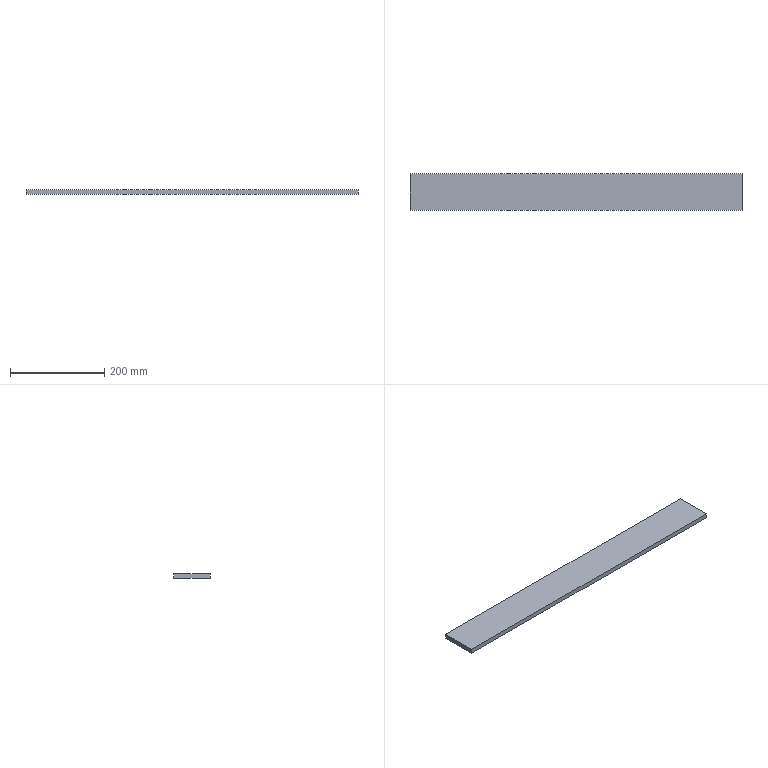Part | STEP file | 06-Square plate | 1 solid | 6 faces | box 703 x 78 x 10 mm | volume 548340 mm3 | plane 6
STEP:
#1=CARTESIAN_POINT('',(0.,0.,0.));
#2=DIRECTION('',(0.,0.,1.));
#3=DIRECTION('',(1.,0.,0.));
#4=AXIS2_PLACEMENT_3D('',#1,#2,#3);
#5=CARTESIAN_POINT('',(0.,0.,0.));
#6=VERTEX_POINT('',#5);
#7=CARTESIAN_POINT('',(0.,-78.,0.));
#8=VERTEX_POINT('',#7);
#9=CARTESIAN_POINT('',(0.,0.,0.));
#10=DIRECTION('',(0.,-1.,0.));
#11=VECTOR('',#10,1.);
#12=LINE('',#9,#11);
#13=CARTESIAN_POINT('',(0.,0.,10.));
#14=DIRECTION('',(1.,0.,0.));
#15=DIRECTION('',(0.,1.,0.));
#16=AXIS2_PLACEMENT_3D('',#13,#14,#15);
#17=PLANE('',#16);
#18=CARTESIAN_POINT('',(0.,-10.));
#19=DIRECTION('',(-1.,0.));
#20=VECTOR('',#19,1.);
#21=LINE('',#18,#20);
#22=(GEOMETRIC_REPRESENTATION_CONTEXT(2)PARAMETRIC_REPRESENTATION_CONTEXT()REPRESENTATION_CONTEXT('',''));
#23=DEFINITIONAL_REPRESENTATION('',(#21),#22);
#24=PCURVE('',#17,#23);
#25=CARTESIAN_POINT('',(0.,0.,0.));
#26=DIRECTION('',(0.,0.,1.));
#27=DIRECTION('',(1.,0.,0.));
#28=AXIS2_PLACEMENT_3D('',#25,#26,#27);
#29=PLANE('',#28);
#30=CARTESIAN_POINT('',(0.,0.));
#31=DIRECTION('',(0.,-1.));
#32=VECTOR('',#31,1.);
#33=LINE('',#30,#32);
#34=(GEOMETRIC_REPRESENTATION_CONTEXT(2)PARAMETRIC_REPRESENTATION_CONTEXT()REPRESENTATION_CONTEXT('',''));
#35=DEFINITIONAL_REPRESENTATION('',(#33),#34);
#36=PCURVE('',#29,#35);
#37=SURFACE_CURVE('',#12,(#24,#36),.PCURVE_S1.);
#38=EDGE_CURVE('',#6,#8,#37,.T.);
#39=ORIENTED_EDGE('',*,*,#38,.T.);
#40=CARTESIAN_POINT('',(0.,-78.,10.));
#41=VERTEX_POINT('',#40);
#42=CARTESIAN_POINT('',(0.,-78.,10.));
#43=DIRECTION('',(0.,0.,-1.));
#44=VECTOR('',#43,1.);
#45=LINE('',#42,#44);
#46=CARTESIAN_POINT('',(-78.,0.));
#47=DIRECTION('',(0.,-1.));
#48=VECTOR('',#47,1.);
#49=LINE('',#46,#48);
#50=(GEOMETRIC_REPRESENTATION_CONTEXT(2)PARAMETRIC_REPRESENTATION_CONTEXT()REPRESENTATION_CONTEXT('',''));
#51=DEFINITIONAL_REPRESENTATION('',(#49),#50);
#52=PCURVE('',#17,#51);
#53=CARTESIAN_POINT('',(0.,-78.,10.));
#54=DIRECTION('',(0.,1.,0.));
#55=DIRECTION('',(0.,0.,1.));
#56=AXIS2_PLACEMENT_3D('',#53,#54,#55);
#57=PLANE('',#56);
#58=CARTESIAN_POINT('',(0.,0.));
#59=DIRECTION('',(-1.,0.));
#60=VECTOR('',#59,1.);
#61=LINE('',#58,#60);
#62=(GEOMETRIC_REPRESENTATION_CONTEXT(2)PARAMETRIC_REPRESENTATION_CONTEXT()REPRESENTATION_CONTEXT('',''));
#63=DEFINITIONAL_REPRESENTATION('',(#61),#62);
#64=PCURVE('',#57,#63);
#65=SURFACE_CURVE('',#45,(#52,#64),.PCURVE_S1.);
#66=EDGE_CURVE('',#41,#8,#65,.T.);
#67=ORIENTED_EDGE('',*,*,#66,.F.);
#68=CARTESIAN_POINT('',(0.,0.,10.));
#69=VERTEX_POINT('',#68);
#70=CARTESIAN_POINT('',(0.,0.,10.));
#71=DIRECTION('',(0.,-1.,0.));
#72=VECTOR('',#71,1.);
#73=LINE('',#70,#72);
#74=CARTESIAN_POINT('',(0.,0.));
#75=DIRECTION('',(-1.,0.));
#76=VECTOR('',#75,1.);
#77=LINE('',#74,#76);
#78=(GEOMETRIC_REPRESENTATION_CONTEXT(2)PARAMETRIC_REPRESENTATION_CONTEXT()REPRESENTATION_CONTEXT('',''));
#79=DEFINITIONAL_REPRESENTATION('',(#77),#78);
#80=PCURVE('',#17,#79);
#81=CARTESIAN_POINT('',(0.,0.,10.));
#82=DIRECTION('',(0.,0.,1.));
#83=DIRECTION('',(1.,0.,0.));
#84=AXIS2_PLACEMENT_3D('',#81,#82,#83);
#85=PLANE('',#84);
#86=CARTESIAN_POINT('',(0.,0.));
#87=DIRECTION('',(0.,-1.));
#88=VECTOR('',#87,1.);
#89=LINE('',#86,#88);
#90=(GEOMETRIC_REPRESENTATION_CONTEXT(2)PARAMETRIC_REPRESENTATION_CONTEXT()REPRESENTATION_CONTEXT('',''));
#91=DEFINITIONAL_REPRESENTATION('',(#89),#90);
#92=PCURVE('',#85,#91);
#93=SURFACE_CURVE('',#73,(#80,#92),.PCURVE_S1.);
#94=EDGE_CURVE('',#69,#41,#93,.T.);
#95=ORIENTED_EDGE('',*,*,#94,.F.);
#96=CARTESIAN_POINT('',(0.,0.,10.));
#97=DIRECTION('',(0.,0.,-1.));
#98=VECTOR('',#97,1.);
#99=LINE('',#96,#98);
#100=CARTESIAN_POINT('',(0.,0.));
#101=DIRECTION('',(0.,-1.));
#102=VECTOR('',#101,1.);
#103=LINE('',#100,#102);
#104=(GEOMETRIC_REPRESENTATION_CONTEXT(2)PARAMETRIC_REPRESENTATION_CONTEXT()REPRESENTATION_CONTEXT('',''));
#105=DEFINITIONAL_REPRESENTATION('',(#103),#104);
#106=PCURVE('',#17,#105);
#107=CARTESIAN_POINT('',(0.,0.,10.));
#108=DIRECTION('',(0.,-1.,0.));
#109=DIRECTION('',(0.,0.,-1.));
#110=AXIS2_PLACEMENT_3D('',#107,#108,#109);
#111=PLANE('',#110);
#112=CARTESIAN_POINT('',(0.,0.));
#113=DIRECTION('',(1.,0.));
#114=VECTOR('',#113,1.);
#115=LINE('',#112,#114);
#116=(GEOMETRIC_REPRESENTATION_CONTEXT(2)PARAMETRIC_REPRESENTATION_CONTEXT()REPRESENTATION_CONTEXT('',''));
#117=DEFINITIONAL_REPRESENTATION('',(#115),#116);
#118=PCURVE('',#111,#117);
#119=SURFACE_CURVE('',#99,(#106,#118),.PCURVE_S1.);
#120=EDGE_CURVE('',#69,#6,#119,.T.);
#121=ORIENTED_EDGE('',*,*,#120,.T.);
#122=EDGE_LOOP('',(#39,#67,#95,#121));
#123=FACE_BOUND('',#122,.T.);
#124=ADVANCED_FACE('',(#123),#17,.F.);
#125=CARTESIAN_POINT('',(703.,-78.,0.));
#126=VERTEX_POINT('',#125);
#127=CARTESIAN_POINT('',(0.,-78.,0.));
#128=DIRECTION('',(1.,0.,0.));
#129=VECTOR('',#128,1.);
#130=LINE('',#127,#129);
#131=CARTESIAN_POINT('',(-10.,0.));
#132=DIRECTION('',(0.,1.));
#133=VECTOR('',#132,1.);
#134=LINE('',#131,#133);
#135=(GEOMETRIC_REPRESENTATION_CONTEXT(2)PARAMETRIC_REPRESENTATION_CONTEXT()REPRESENTATION_CONTEXT('',''));
#136=DEFINITIONAL_REPRESENTATION('',(#134),#135);
#137=PCURVE('',#57,#136);
#138=CARTESIAN_POINT('',(0.,-78.));
#139=DIRECTION('',(1.,0.));
#140=VECTOR('',#139,1.);
#141=LINE('',#138,#140);
#142=(GEOMETRIC_REPRESENTATION_CONTEXT(2)PARAMETRIC_REPRESENTATION_CONTEXT()REPRESENTATION_CONTEXT('',''));
#143=DEFINITIONAL_REPRESENTATION('',(#141),#142);
#144=PCURVE('',#29,#143);
#145=SURFACE_CURVE('',#130,(#137,#144),.PCURVE_S1.);
#146=EDGE_CURVE('',#8,#126,#145,.T.);
#147=ORIENTED_EDGE('',*,*,#146,.T.);
#148=CARTESIAN_POINT('',(703.,-78.,10.));
#149=VERTEX_POINT('',#148);
#150=CARTESIAN_POINT('',(703.,-78.,10.));
#151=DIRECTION('',(0.,0.,-1.));
#152=VECTOR('',#151,1.);
#153=LINE('',#150,#152);
#154=CARTESIAN_POINT('',(0.,703.));
#155=DIRECTION('',(-1.,0.));
#156=VECTOR('',#155,1.);
#157=LINE('',#154,#156);
#158=(GEOMETRIC_REPRESENTATION_CONTEXT(2)PARAMETRIC_REPRESENTATION_CONTEXT()REPRESENTATION_CONTEXT('',''));
#159=DEFINITIONAL_REPRESENTATION('',(#157),#158);
#160=PCURVE('',#57,#159);
#161=CARTESIAN_POINT('',(703.,0.,10.));
#162=DIRECTION('',(-1.,0.,0.));
#163=DIRECTION('',(0.,-1.,0.));
#164=AXIS2_PLACEMENT_3D('',#161,#162,#163);
#165=PLANE('',#164);
#166=CARTESIAN_POINT('',(78.,0.));
#167=DIRECTION('',(0.,-1.));
#168=VECTOR('',#167,1.);
#169=LINE('',#166,#168);
#170=(GEOMETRIC_REPRESENTATION_CONTEXT(2)PARAMETRIC_REPRESENTATION_CONTEXT()REPRESENTATION_CONTEXT('',''));
#171=DEFINITIONAL_REPRESENTATION('',(#169),#170);
#172=PCURVE('',#165,#171);
#173=SURFACE_CURVE('',#153,(#160,#172),.PCURVE_S1.);
#174=EDGE_CURVE('',#149,#126,#173,.T.);
#175=ORIENTED_EDGE('',*,*,#174,.F.);
#176=CARTESIAN_POINT('',(0.,-78.,10.));
#177=DIRECTION('',(1.,0.,0.));
#178=VECTOR('',#177,1.);
#179=LINE('',#176,#178);
#180=CARTESIAN_POINT('',(0.,0.));
#181=DIRECTION('',(0.,1.));
#182=VECTOR('',#181,1.);
#183=LINE('',#180,#182);
#184=(GEOMETRIC_REPRESENTATION_CONTEXT(2)PARAMETRIC_REPRESENTATION_CONTEXT()REPRESENTATION_CONTEXT('',''));
#185=DEFINITIONAL_REPRESENTATION('',(#183),#184);
#186=PCURVE('',#57,#185);
#187=CARTESIAN_POINT('',(0.,-78.));
#188=DIRECTION('',(1.,0.));
#189=VECTOR('',#188,1.);
#190=LINE('',#187,#189);
#191=(GEOMETRIC_REPRESENTATION_CONTEXT(2)PARAMETRIC_REPRESENTATION_CONTEXT()REPRESENTATION_CONTEXT('',''));
#192=DEFINITIONAL_REPRESENTATION('',(#190),#191);
#193=PCURVE('',#85,#192);
#194=SURFACE_CURVE('',#179,(#186,#193),.PCURVE_S1.);
#195=EDGE_CURVE('',#41,#149,#194,.T.);
#196=ORIENTED_EDGE('',*,*,#195,.F.);
#197=ORIENTED_EDGE('',*,*,#66,.T.);
#198=EDGE_LOOP('',(#147,#175,#196,#197));
#199=FACE_BOUND('',#198,.T.);
#200=ADVANCED_FACE('',(#199),#57,.F.);
#201=CARTESIAN_POINT('',(703.,0.,0.));
#202=VERTEX_POINT('',#201);
#203=CARTESIAN_POINT('',(703.,0.,0.));
#204=DIRECTION('',(0.,1.,0.));
#205=VECTOR('',#204,1.);
#206=LINE('',#203,#205);
#207=CARTESIAN_POINT('',(0.,-10.));
#208=DIRECTION('',(-1.,0.));
#209=VECTOR('',#208,1.);
#210=LINE('',#207,#209);
#211=(GEOMETRIC_REPRESENTATION_CONTEXT(2)PARAMETRIC_REPRESENTATION_CONTEXT()REPRESENTATION_CONTEXT('',''));
#212=DEFINITIONAL_REPRESENTATION('',(#210),#211);
#213=PCURVE('',#165,#212);
#214=CARTESIAN_POINT('',(703.,0.));
#215=DIRECTION('',(0.,1.));
#216=VECTOR('',#215,1.);
#217=LINE('',#214,#216);
#218=(GEOMETRIC_REPRESENTATION_CONTEXT(2)PARAMETRIC_REPRESENTATION_CONTEXT()REPRESENTATION_CONTEXT('',''));
#219=DEFINITIONAL_REPRESENTATION('',(#217),#218);
#220=PCURVE('',#29,#219);
#221=SURFACE_CURVE('',#206,(#213,#220),.PCURVE_S1.);
#222=EDGE_CURVE('',#126,#202,#221,.T.);
#223=ORIENTED_EDGE('',*,*,#222,.T.);
#224=CARTESIAN_POINT('',(703.,0.,10.));
#225=VERTEX_POINT('',#224);
#226=CARTESIAN_POINT('',(703.,0.,10.));
#227=DIRECTION('',(0.,0.,-1.));
#228=VECTOR('',#227,1.);
#229=LINE('',#226,#228);
#230=CARTESIAN_POINT('',(0.,0.));
#231=DIRECTION('',(0.,-1.));
#232=VECTOR('',#231,1.);
#233=LINE('',#230,#232);
#234=(GEOMETRIC_REPRESENTATION_CONTEXT(2)PARAMETRIC_REPRESENTATION_CONTEXT()REPRESENTATION_CONTEXT('',''));
#235=DEFINITIONAL_REPRESENTATION('',(#233),#234);
#236=PCURVE('',#165,#235);
#237=CARTESIAN_POINT('',(0.,703.));
#238=DIRECTION('',(1.,0.));
#239=VECTOR('',#238,1.);
#240=LINE('',#237,#239);
#241=(GEOMETRIC_REPRESENTATION_CONTEXT(2)PARAMETRIC_REPRESENTATION_CONTEXT()REPRESENTATION_CONTEXT('',''));
#242=DEFINITIONAL_REPRESENTATION('',(#240),#241);
#243=PCURVE('',#111,#242);
#244=SURFACE_CURVE('',#229,(#236,#243),.PCURVE_S1.);
#245=EDGE_CURVE('',#225,#202,#244,.T.);
#246=ORIENTED_EDGE('',*,*,#245,.F.);
#247=CARTESIAN_POINT('',(703.,0.,10.));
#248=DIRECTION('',(0.,1.,0.));
#249=VECTOR('',#248,1.);
#250=LINE('',#247,#249);
#251=CARTESIAN_POINT('',(0.,0.));
#252=DIRECTION('',(-1.,0.));
#253=VECTOR('',#252,1.);
#254=LINE('',#251,#253);
#255=(GEOMETRIC_REPRESENTATION_CONTEXT(2)PARAMETRIC_REPRESENTATION_CONTEXT()REPRESENTATION_CONTEXT('',''));
#256=DEFINITIONAL_REPRESENTATION('',(#254),#255);
#257=PCURVE('',#165,#256);
#258=CARTESIAN_POINT('',(703.,0.));
#259=DIRECTION('',(0.,1.));
#260=VECTOR('',#259,1.);
#261=LINE('',#258,#260);
#262=(GEOMETRIC_REPRESENTATION_CONTEXT(2)PARAMETRIC_REPRESENTATION_CONTEXT()REPRESENTATION_CONTEXT('',''));
#263=DEFINITIONAL_REPRESENTATION('',(#261),#262);
#264=PCURVE('',#85,#263);
#265=SURFACE_CURVE('',#250,(#257,#264),.PCURVE_S1.);
#266=EDGE_CURVE('',#149,#225,#265,.T.);
#267=ORIENTED_EDGE('',*,*,#266,.F.);
#268=ORIENTED_EDGE('',*,*,#174,.T.);
#269=EDGE_LOOP('',(#223,#246,#267,#268));
#270=FACE_BOUND('',#269,.T.);
#271=ADVANCED_FACE('',(#270),#165,.F.);
#272=CARTESIAN_POINT('',(0.,0.,0.));
#273=DIRECTION('',(-1.,0.,0.));
#274=VECTOR('',#273,1.);
#275=LINE('',#272,#274);
#276=CARTESIAN_POINT('',(10.,0.));
#277=DIRECTION('',(0.,-1.));
#278=VECTOR('',#277,1.);
#279=LINE('',#276,#278);
#280=(GEOMETRIC_REPRESENTATION_CONTEXT(2)PARAMETRIC_REPRESENTATION_CONTEXT()REPRESENTATION_CONTEXT('',''));
#281=DEFINITIONAL_REPRESENTATION('',(#279),#280);
#282=PCURVE('',#111,#281);
#283=CARTESIAN_POINT('',(0.,0.));
#284=DIRECTION('',(-1.,0.));
#285=VECTOR('',#284,1.);
#286=LINE('',#283,#285);
#287=(GEOMETRIC_REPRESENTATION_CONTEXT(2)PARAMETRIC_REPRESENTATION_CONTEXT()REPRESENTATION_CONTEXT('',''));
#288=DEFINITIONAL_REPRESENTATION('',(#286),#287);
#289=PCURVE('',#29,#288);
#290=SURFACE_CURVE('',#275,(#282,#289),.PCURVE_S1.);
#291=EDGE_CURVE('',#202,#6,#290,.T.);
#292=ORIENTED_EDGE('',*,*,#291,.T.);
#293=ORIENTED_EDGE('',*,*,#120,.F.);
#294=CARTESIAN_POINT('',(0.,0.,10.));
#295=DIRECTION('',(-1.,0.,0.));
#296=VECTOR('',#295,1.);
#297=LINE('',#294,#296);
#298=CARTESIAN_POINT('',(0.,0.));
#299=DIRECTION('',(0.,-1.));
#300=VECTOR('',#299,1.);
#301=LINE('',#298,#300);
#302=(GEOMETRIC_REPRESENTATION_CONTEXT(2)PARAMETRIC_REPRESENTATION_CONTEXT()REPRESENTATION_CONTEXT('',''));
#303=DEFINITIONAL_REPRESENTATION('',(#301),#302);
#304=PCURVE('',#111,#303);
#305=CARTESIAN_POINT('',(0.,0.));
#306=DIRECTION('',(-1.,0.));
#307=VECTOR('',#306,1.);
#308=LINE('',#305,#307);
#309=(GEOMETRIC_REPRESENTATION_CONTEXT(2)PARAMETRIC_REPRESENTATION_CONTEXT()REPRESENTATION_CONTEXT('',''));
#310=DEFINITIONAL_REPRESENTATION('',(#308),#309);
#311=PCURVE('',#85,#310);
#312=SURFACE_CURVE('',#297,(#304,#311),.PCURVE_S1.);
#313=EDGE_CURVE('',#225,#69,#312,.T.);
#314=ORIENTED_EDGE('',*,*,#313,.F.);
#315=ORIENTED_EDGE('',*,*,#245,.T.);
#316=EDGE_LOOP('',(#292,#293,#314,#315));
#317=FACE_BOUND('',#316,.T.);
#318=ADVANCED_FACE('',(#317),#111,.F.);
#319=ORIENTED_EDGE('',*,*,#94,.T.);
#320=ORIENTED_EDGE('',*,*,#195,.T.);
#321=ORIENTED_EDGE('',*,*,#266,.T.);
#322=ORIENTED_EDGE('',*,*,#313,.T.);
#323=EDGE_LOOP('',(#319,#320,#321,#322));
#324=FACE_BOUND('',#323,.T.);
#325=ADVANCED_FACE('',(#324),#85,.T.);
#326=ORIENTED_EDGE('',*,*,#38,.F.);
#327=ORIENTED_EDGE('',*,*,#291,.F.);
#328=ORIENTED_EDGE('',*,*,#222,.F.);
#329=ORIENTED_EDGE('',*,*,#146,.F.);
#330=EDGE_LOOP('',(#326,#327,#328,#329));
#331=FACE_BOUND('',#330,.T.);
#332=ADVANCED_FACE('',(#331),#29,.F.);
#333=CLOSED_SHELL('',(#124,#200,#271,#318,#325,#332));
#334=MANIFOLD_SOLID_BREP('',#333);
#335=(LENGTH_UNIT()NAMED_UNIT(*)SI_UNIT(.MILLI.,.METRE.));
#336=UNCERTAINTY_MEASURE_WITH_UNIT(LENGTH_MEASURE(0.0000001),#335,'','');
#337=(NAMED_UNIT(*)PLANE_ANGLE_UNIT()SI_UNIT($,.RADIAN.));
#338=(NAMED_UNIT(*)SI_UNIT($,.STERADIAN.)SOLID_ANGLE_UNIT());
#339=(GEOMETRIC_REPRESENTATION_CONTEXT(3)GLOBAL_UNCERTAINTY_ASSIGNED_CONTEXT((#336))GLOBAL_UNIT_ASSIGNED_CONTEXT((#335,#337,#338))REPRESENTATION_CONTEXT('',''));
#340=ADVANCED_BREP_SHAPE_REPRESENTATION('',(#4,#334),#339);